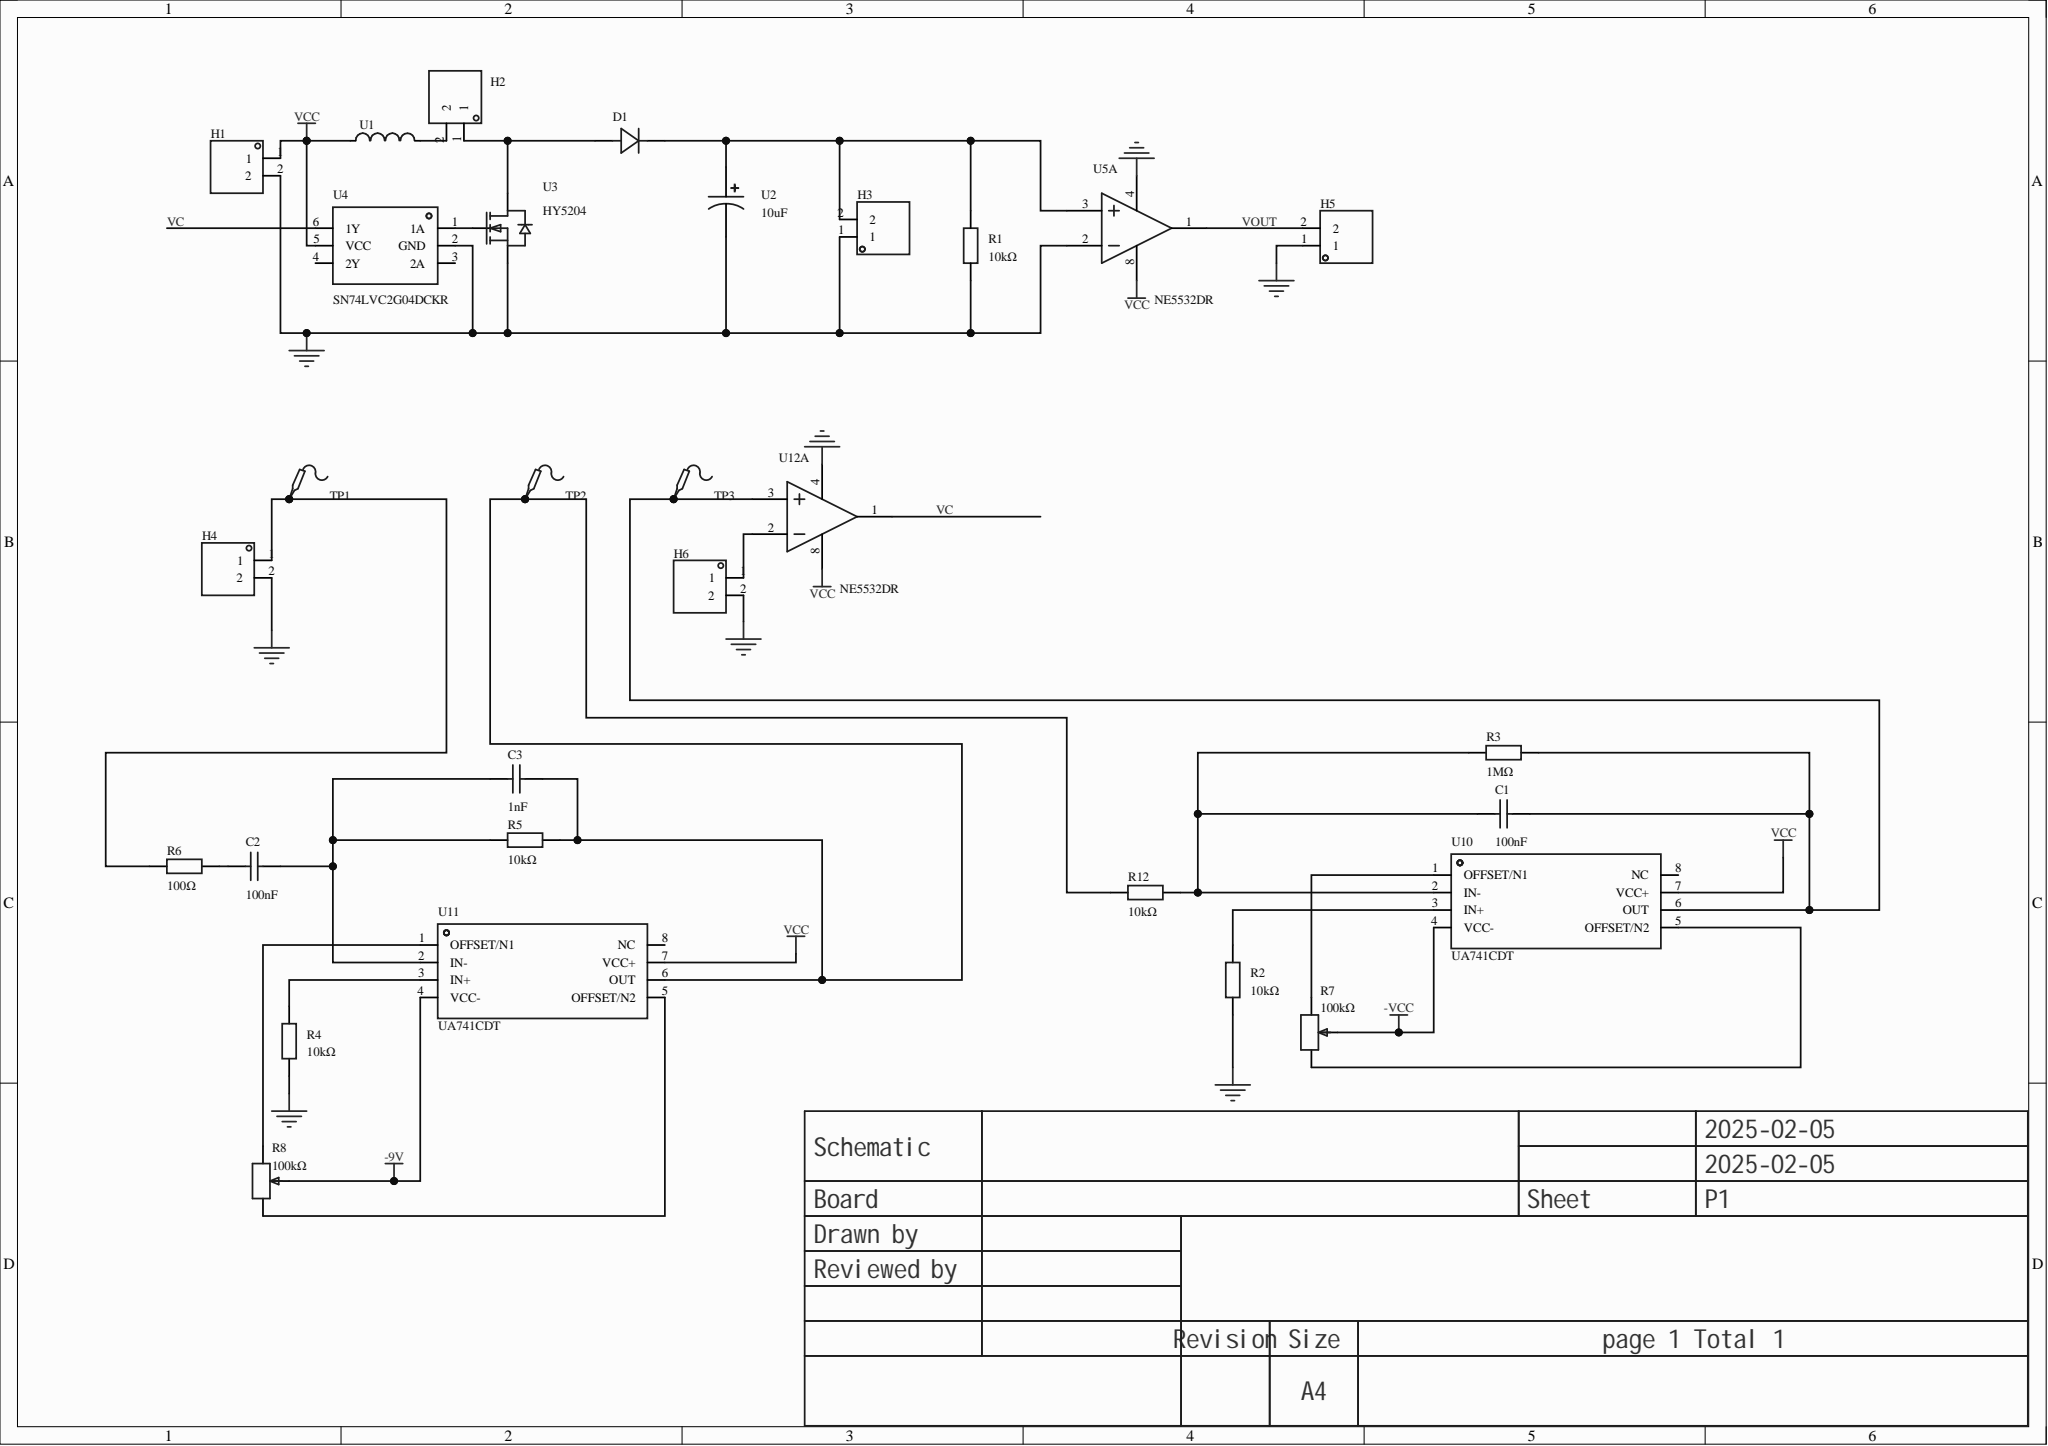Circuit board | Altium Designer | 30 parts | 23 nets
Bill of materials:
Comment,Description,Designator,Footprint,LibRef,Quantity
"100nF","Capacitance:100nF;Tolerance:±10%;Rated voltage:50V;Material (temperature coefficient):X7R;","C1, C2","C0805","CC0805KRX7R9BB104","2"
"1nF","Capacitance:100nF;Tolerance:±10%;Rated voltage:50V;Material (temperature coefficient):X7R;","C3","C0805","CC0805KRX7R9BB104","1"
"","","D1","DO_1N4007","D_1N4007A","1"
"","","H1, H2, H3, H4, H5, H6","HDR-TH_2P-P2.54-V-M-1","HDR-M_2.54_1x2P","6"
"10kΩ","","R1","Res_1/4W","Res_AXIAL-1/4W","1"
"10kΩ","Resistor type:Thick film resistor;Resistance:10kΩ;Tolerance:±1%;Power:125mW;Max working voltage:150V;Temperature coefficient:±100ppm/?;","R2, R4, R5, R12","R0805","0805W8F1002T5E_C17414","4"
"1MΩ","Resistor type:Thick film resistor;Resistance:10kΩ;Tolerance:±1%;Power:125mW;Max working voltage:150V;Temperature coefficient:±100ppm/?;","R3","R0805","0805W8F1002T5E_C17414","1"
"100Ω","Resistor type:Thick film resistor;Resistance:10kΩ;Tolerance:±1%;Power:125mW;Max working voltage:150V;Temperature coefficient:±100ppm/?;","R6","R0805","0805W8F1002T5E_C17414","1"
"100kΩ","Resistance:200Ω;Tolerance:±25%;","R7, R8","RES-ADJ-SMD_VG039NCH","VG039NCHXTB201","2"
"","Test Point","TP1, TP2, TP3","Test-Point-0.5mm","Test-Point","3"
"Power inductor (SMD),CKST0502-10uH/M,10uH,±20%,3A,package 5.7mm*5.1mm*2.0mm,CENKER,RoHS","","U1","IND-SMD_L5.7-W5.1","功率电感(贴片),CKST0502-10uH/M,10uH,±20%,3A,封装5.7mm*5.1mm*2.0mm,岑科,RoHS","1"
"10uF","Capacitance:10uF;Tolerance:±20%;Rated voltage:10V;Ripple current:16mA@120Hz;","U2","CAP-TH_BD4.0-P1.50-D0.8-FD","10MS510MEFC4X5","1"
"HY5204","","U3","TO-247-3_L15.8-W5.0-P5.44-L-1","HY5204","1"
"SN74LVC2G04DCKR","Input type:-;Supply voltage:1.65V~5.5V;Supply current (max):10uA;Number of circuits:2;Max propagation delay (tpd):3.2ns@5V,50pF;","U4","SOT-363_L2.0-W1.3-P0.65-LS2.1-BR","SN74LVC2G04DCKR","1"
"NE5532DR","Number of amplifiers:Dual;Gain bandwidth product (GBP):10MHz;Input bias current (Ib):200nA;Slew rate (SR):9V/us;Bandwidth (-3db):-;","U5, U12","SOIC-8_L4.9-W3.9-P1.27-LS6.0-BL","NE5532DR","2"
"UA741CDT","Number of amplifiers:Single;Gain bandwidth product (GBP):1MHz;Input bias current (Ib):10nA;Slew rate (SR):0.5V/us;Bandwidth (-3db):-;","U10, U11","SOIC-8_L4.9-W3.9-P1.27-LS6.0-BL","UA741CDT","2"
Netlist (Protel format):
[
C1
C0805
100nF



]
[
C2
C0805
100nF



]
[
C3
C0805
1nF



]
[
D1
DO_1N4007




]
[
H1
HDR-TH_2P-P2.54-V-M-1




]
[
H2
HDR-TH_2P-P2.54-V-M-1




]
[
H3
HDR-TH_2P-P2.54-V-M-1




]
[
H4
HDR-TH_2P-P2.54-V-M-1




]
[
H5
HDR-TH_2P-P2.54-V-M-1




]
[
H6
HDR-TH_2P-P2.54-V-M-1




]
[
R1
Res_1/4W
10kΩ



]
[
R2
R0805
10kΩ



]
[
R3
R0805
1MΩ



]
[
R4
R0805
10kΩ



]
[
R5
R0805
10kΩ



]
[
R6
R0805
100Ω



]
[
R7
RES-ADJ-SMD_VG039NCH
100kΩ



]
[
R8
RES-ADJ-SMD_VG039NCH
100kΩ



]
[
R12
R0805
10kΩ



]
[
TP1
Test-Point-0.5mm




]
[
TP2
Test-Point-0.5mm




]
[
TP3
Test-Point-0.5mm




]
[
U1
IND-SMD_L5.7-W5.1
Power inductor (SMD),CKST0502-10uH/M,10uH,±20%,3A,package 5.7mm*5.1mm*2.0mm,CENKER,RoHS



]
[
U2
CAP-TH_BD4.0-P1.50-D0.8-FD
10uF



]
[
U3
TO-247-3_L15.8-W5.0-P5.44-L-1
HY5204



]
[
U4
SOT-363_L2.0-W1.3-P0.65-LS2.1-BR
SN74LVC2G04DCKR



]
[
U5
SOIC-8_L4.9-W3.9-P1.27-LS6.0-BL
NE5532DR



]
[
U10
SOIC-8_L4.9-W3.9-P1.27-LS6.0-BL
UA741CDT



]
[
U11
SOIC-8_L4.9-W3.9-P1.27-LS6.0-BL
UA741CDT



]
[
U12
SOIC-8_L4.9-W3.9-P1.27-LS6.0-BL
NE5532DR



]
(
VOUT
H5-2
U5-1
)
(
VCC
H1-1
U1-1
U4-5
U5-8
U10-7
U11-7
U12-8
)
(
VC
U4-6
U12-1
)
(
NetU3_1
U3-1
U4-1
)
(
NetR8_3
R8-3
U11-5
)
(
NetR8_1
R8-1
U11-1
)
(
NetR7_3
R7-3
U10-1
)
(
NetR7_1
R7-1
U10-5
)
(
NetR4_2
R4-2
U11-3
)
(
NetR2_2
R2-2
U10-3
)
(
NetH6_1
H6-1
U12-2
)
(
NetH4_1
H4-1
R6-1
TP1-1
)
(
NetH2_2
H2-2
U1-2
)
(
NetD1_2
D1-2
H2-1
U3-2
)
(
NetD1_1
D1-1
H3-2
R1-2
U2-1
U5-3
)
(
NetC3_2
C3-2
R5-2
R12-1
TP2-1
U11-6
)
(
NetC2_2
C2-2
C3-1
R5-1
U11-2
)
(
NetC2_1
C2-1
R6-2
)
(
NetC1_2
C1-2
R3-2
TP3-1
U10-6
U12-3
)
(
NetC1_1
C1-1
R3-1
R12-2
U10-2
)
(
GND
H1-2
H3-1
H4-2
H5-1
H6-2
R1-1
R2-1
R4-1
U2-2
U3-3
U4-2
U5-2
U5-4
U12-4
)
(
-VCC
R7-2
U10-4
)
(
-9V
R8-2
U11-4
)